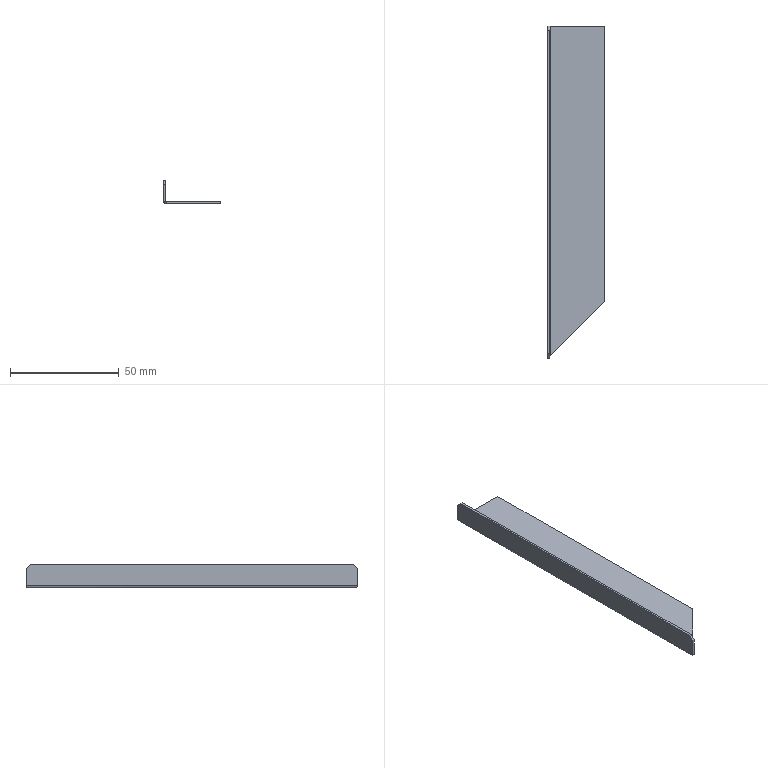Part | SolidWorks | features Chamfer 1, SplitBody 1 | 1 solid | 16 faces | box 26 x 152.414 x 11 mm | volume 5106 mm3 | plane 13 | cylinder 2 | spline 1 | commonest cylinder face diameters 0.2 x1 2.2 x1
STEP:
#1=CARTESIAN_POINT('',(-547.9,348.,56.));
#2=VERTEX_POINT('',#1);
#3=CARTESIAN_POINT('',(-547.9,348.,55.));
#4=VERTEX_POINT('',#3);
#5=CARTESIAN_POINT('',(-547.9,348.,56.));
#6=DIRECTION('',(0.,0.,-1.));
#7=VECTOR('',#6,1000.);
#8=LINE('',#5,#7);
#9=EDGE_CURVE('',#2,#4,#8,.T.);
#10=ORIENTED_EDGE('',*,*,#9,.F.);
#11=CARTESIAN_POINT('',(-523.,348.,56.));
#12=VERTEX_POINT('',#11);
#13=CARTESIAN_POINT('',(-549.,348.,56.));
#14=DIRECTION('',(1.,0.,0.));
#15=VECTOR('',#14,1000.);
#16=LINE('',#13,#15);
#17=EDGE_CURVE('',#2,#12,#16,.T.);
#18=ORIENTED_EDGE('',*,*,#17,.T.);
#19=CARTESIAN_POINT('',(-523.,348.,55.));
#20=VERTEX_POINT('',#19);
#21=CARTESIAN_POINT('',(-523.,348.,56.));
#22=DIRECTION('',(0.,0.,-1.));
#23=VECTOR('',#22,1000.);
#24=LINE('',#21,#23);
#25=EDGE_CURVE('',#12,#20,#24,.T.);
#26=ORIENTED_EDGE('',*,*,#25,.T.);
#27=CARTESIAN_POINT('',(-549.,348.,55.));
#28=DIRECTION('',(1.,0.,0.));
#29=VECTOR('',#28,1000.);
#30=LINE('',#27,#29);
#31=EDGE_CURVE('',#4,#20,#30,.T.);
#32=ORIENTED_EDGE('',*,*,#31,.F.);
#33=EDGE_LOOP('',(#10,#18,#26,#32));
#34=FACE_OUTER_BOUND('',#33,.T.);
#35=CARTESIAN_POINT('',(-549.,348.,56.));
#36=DIRECTION('',(0.,-1.,0.));
#37=DIRECTION('',(0.,0.,1.));
#38=AXIS2_PLACEMENT_3D('',#35,#36,#37);
#39=PLANE('',#38);
#40=ADVANCED_FACE('',(#34),#39,.F.);
#41=CARTESIAN_POINT('',(-547.9,196.686,56.));
#42=VERTEX_POINT('',#41);
#43=CARTESIAN_POINT('',(-547.9,196.686,55.));
#44=VERTEX_POINT('',#43);
#45=CARTESIAN_POINT('',(-547.9,196.686,56.));
#46=DIRECTION('',(0.,0.,-1.));
#47=VECTOR('',#46,1000.);
#48=LINE('',#45,#47);
#49=EDGE_CURVE('',#42,#44,#48,.T.);
#50=ORIENTED_EDGE('',*,*,#49,.T.);
#51=CARTESIAN_POINT('',(-523.,221.586,55.));
#52=VERTEX_POINT('',#51);
#53=CARTESIAN_POINT('',(-523.,221.586,55.));
#54=DIRECTION('',(-0.7071,-0.7071,0.));
#55=VECTOR('',#54,1000.);
#56=LINE('',#53,#55);
#57=EDGE_CURVE('',#52,#44,#56,.T.);
#58=ORIENTED_EDGE('',*,*,#57,.F.);
#59=CARTESIAN_POINT('',(-523.,221.586,56.));
#60=VERTEX_POINT('',#59);
#61=CARTESIAN_POINT('',(-523.,221.586,56.));
#62=DIRECTION('',(0.,0.,-1.));
#63=VECTOR('',#62,1000.);
#64=LINE('',#61,#63);
#65=EDGE_CURVE('',#60,#52,#64,.T.);
#66=ORIENTED_EDGE('',*,*,#65,.F.);
#67=CARTESIAN_POINT('',(-523.,221.586,56.));
#68=DIRECTION('',(-0.7071,-0.7071,0.));
#69=VECTOR('',#68,1000.);
#70=LINE('',#67,#69);
#71=EDGE_CURVE('',#60,#42,#70,.T.);
#72=ORIENTED_EDGE('',*,*,#71,.T.);
#73=EDGE_LOOP('',(#50,#58,#66,#72));
#74=FACE_OUTER_BOUND('',#73,.T.);
#75=CARTESIAN_POINT('',(-523.,221.586,56.));
#76=DIRECTION('',(-0.7071,0.7071,0.));
#77=DIRECTION('',(-0.7071,-0.7071,0.));
#78=AXIS2_PLACEMENT_3D('',#75,#76,#77);
#79=PLANE('',#78);
#80=ADVANCED_FACE('',(#74),#79,.F.);
#81=ORIENTED_EDGE('',*,*,#71,.F.);
#82=CARTESIAN_POINT('',(-523.,348.,56.));
#83=DIRECTION('',(0.,-1.,0.));
#84=VECTOR('',#83,1000.);
#85=LINE('',#82,#84);
#86=EDGE_CURVE('',#12,#60,#85,.T.);
#87=ORIENTED_EDGE('',*,*,#86,.F.);
#88=ORIENTED_EDGE('',*,*,#17,.F.);
#89=CARTESIAN_POINT('',(-547.9,348.,56.));
#90=DIRECTION('',(0.,-1.,0.));
#91=VECTOR('',#90,1000.);
#92=LINE('',#89,#91);
#93=EDGE_CURVE('',#2,#42,#92,.T.);
#94=ORIENTED_EDGE('',*,*,#93,.T.);
#95=EDGE_LOOP('',(#81,#87,#88,#94));
#96=FACE_OUTER_BOUND('',#95,.T.);
#97=CARTESIAN_POINT('',(0.,0.,56.));
#98=DIRECTION('',(0.,0.,1.));
#99=DIRECTION('',(0.,1.,0.));
#100=AXIS2_PLACEMENT_3D('',#97,#98,#99);
#101=PLANE('',#100);
#102=ADVANCED_FACE('',(#96),#101,.T.);
#103=CARTESIAN_POINT('',(-547.9,348.,55.));
#104=DIRECTION('',(0.,-1.,0.));
#105=VECTOR('',#104,1000.);
#106=LINE('',#103,#105);
#107=EDGE_CURVE('',#4,#44,#106,.T.);
#108=ORIENTED_EDGE('',*,*,#107,.F.);
#109=ORIENTED_EDGE('',*,*,#31,.T.);
#110=CARTESIAN_POINT('',(-523.,348.,55.));
#111=DIRECTION('',(0.,-1.,0.));
#112=VECTOR('',#111,1000.);
#113=LINE('',#110,#112);
#114=EDGE_CURVE('',#20,#52,#113,.T.);
#115=ORIENTED_EDGE('',*,*,#114,.T.);
#116=ORIENTED_EDGE('',*,*,#57,.T.);
#117=EDGE_LOOP('',(#108,#109,#115,#116));
#118=FACE_OUTER_BOUND('',#117,.T.);
#119=CARTESIAN_POINT('',(0.,0.,55.));
#120=DIRECTION('',(0.,0.,1.));
#121=DIRECTION('',(0.,1.,0.));
#122=AXIS2_PLACEMENT_3D('',#119,#120,#121);
#123=PLANE('',#122);
#124=ADVANCED_FACE('',(#118),#123,.F.);
#125=ORIENTED_EDGE('',*,*,#114,.F.);
#126=ORIENTED_EDGE('',*,*,#25,.F.);
#127=ORIENTED_EDGE('',*,*,#86,.T.);
#128=ORIENTED_EDGE('',*,*,#65,.T.);
#129=EDGE_LOOP('',(#125,#126,#127,#128));
#130=FACE_OUTER_BOUND('',#129,.T.);
#131=CARTESIAN_POINT('',(-523.,348.,56.));
#132=DIRECTION('',(-1.,0.,0.));
#133=DIRECTION('',(0.,0.,-1.));
#134=AXIS2_PLACEMENT_3D('',#131,#132,#133);
#135=PLANE('',#134);
#136=ADVANCED_FACE('',(#130),#135,.F.);
#137=CARTESIAN_POINT('',(-548.,195.586,56.1));
#138=VERTEX_POINT('',#137);
#139=CARTESIAN_POINT('',(-549.,195.586,56.1));
#140=VERTEX_POINT('',#139);
#141=CARTESIAN_POINT('',(-549.,195.586,56.1));
#142=DIRECTION('',(-1.,0.,0.));
#143=VECTOR('',#142,1000.);
#144=LINE('',#141,#143);
#145=EDGE_CURVE('',#138,#140,#144,.T.);
#146=ORIENTED_EDGE('',*,*,#145,.T.);
#147=CARTESIAN_POINT('',(-547.9,196.686,55.));
#148=CARTESIAN_POINT('',(-548.191,196.501,55.));
#149=CARTESIAN_POINT('',(-548.473,196.32,55.117));
#150=CARTESIAN_POINT('',(-548.781,196.043,55.425));
#151=CARTESIAN_POINT('',(-548.861,195.953,55.545));
#152=CARTESIAN_POINT('',(-548.972,195.768,55.813));
#153=CARTESIAN_POINT('',(-549.,195.678,55.955));
#154=CARTESIAN_POINT('',(-549.,195.586,56.1));
#155=B_SPLINE_CURVE_WITH_KNOTS('',3,(#147,#148,#149,#150,#151,#152,#153,#154),.UNSPECIFIED.,.F.,.F.,(4,2,2,4),(0.,0.001021,0.001531,0.002041),.UNSPECIFIED.);
#156=EDGE_CURVE('',#44,#140,#155,.T.);
#157=ORIENTED_EDGE('',*,*,#156,.F.);
#158=ORIENTED_EDGE('',*,*,#49,.F.);
#159=CARTESIAN_POINT('',(-547.9,196.686,56.));
#160=CARTESIAN_POINT('',(-547.926,196.502,56.));
#161=CARTESIAN_POINT('',(-547.952,196.319,56.011));
#162=CARTESIAN_POINT('',(-547.989,195.952,56.048));
#163=CARTESIAN_POINT('',(-548.,195.769,56.074));
#164=CARTESIAN_POINT('',(-548.,195.586,56.1));
#165=B_SPLINE_CURVE_WITH_KNOTS('',3,(#159,#160,#161,#162,#163,#164),.UNSPECIFIED.,.F.,.F.,(4,2,4),(0.,0.5,1.),.UNSPECIFIED.);
#166=EDGE_CURVE('',#42,#138,#165,.T.);
#167=ORIENTED_EDGE('',*,*,#166,.T.);
#168=EDGE_LOOP('',(#146,#157,#158,#167));
#169=FACE_OUTER_BOUND('',#168,.T.);
#170=CARTESIAN_POINT('',(-547.9,196.686,54.99));
#171=CARTESIAN_POINT('',(-548.045,196.594,54.99));
#172=CARTESIAN_POINT('',(-548.191,196.502,55.019));
#173=CARTESIAN_POINT('',(-548.459,196.319,55.13));
#174=CARTESIAN_POINT('',(-548.582,196.227,55.212));
#175=CARTESIAN_POINT('',(-548.788,196.044,55.418));
#176=CARTESIAN_POINT('',(-548.87,195.952,55.541));
#177=CARTESIAN_POINT('',(-548.981,195.769,55.809));
#178=CARTESIAN_POINT('',(-549.01,195.677,55.955));
#179=CARTESIAN_POINT('',(-549.01,195.586,56.1));
#180=CARTESIAN_POINT('',(-547.9,196.686,55.));
#181=CARTESIAN_POINT('',(-548.044,196.594,55.));
#182=CARTESIAN_POINT('',(-548.188,196.502,55.029));
#183=CARTESIAN_POINT('',(-548.454,196.319,55.139));
#184=CARTESIAN_POINT('',(-548.576,196.227,55.22));
#185=CARTESIAN_POINT('',(-548.78,196.044,55.424));
#186=CARTESIAN_POINT('',(-548.861,195.952,55.546));
#187=CARTESIAN_POINT('',(-548.971,195.769,55.812));
#188=CARTESIAN_POINT('',(-549.,195.677,55.956));
#189=CARTESIAN_POINT('',(-549.,195.586,56.1));
#190=CARTESIAN_POINT('',(-547.9,196.686,56.));
#191=CARTESIAN_POINT('',(-547.913,196.594,56.));
#192=CARTESIAN_POINT('',(-547.926,196.502,56.003));
#193=CARTESIAN_POINT('',(-547.95,196.319,56.013));
#194=CARTESIAN_POINT('',(-547.961,196.227,56.02));
#195=CARTESIAN_POINT('',(-547.98,196.044,56.039));
#196=CARTESIAN_POINT('',(-547.987,195.952,56.05));
#197=CARTESIAN_POINT('',(-547.997,195.769,56.074));
#198=CARTESIAN_POINT('',(-548.,195.677,56.087));
#199=CARTESIAN_POINT('',(-548.,195.586,56.1));
#200=B_SPLINE_SURFACE_WITH_KNOTS('',1,3,((#170,#171,#172,#173,#174,#175,#176,#177,#178,#179),(#180,#181,#182,#183,#184,#185,#186,#187,#188,#189),(#190,#191,#192,#193,#194,#195,#196,#197,#198,#199)),.UNSPECIFIED.,.F.,.F.,.F.,(2,1,2),(4,2,2,2,4),(-0.01,0.,1.),(0.,0.25,0.5,0.75,1.),.UNSPECIFIED.);
#201=ADVANCED_FACE('',(#169),#200,.T.);
#202=CARTESIAN_POINT('',(-548.,348.,56.1));
#203=VERTEX_POINT('',#202);
#204=CARTESIAN_POINT('',(-547.9,348.,56.1));
#205=DIRECTION('',(0.,-1.,0.));
#206=DIRECTION('',(0.,0.,-1.));
#207=AXIS2_PLACEMENT_3D('',#204,#205,#206);
#208=CIRCLE('',#207,0.1);
#209=EDGE_CURVE('',#203,#2,#208,.T.);
#210=ORIENTED_EDGE('',*,*,#209,.T.);
#211=ORIENTED_EDGE('',*,*,#9,.T.);
#212=CARTESIAN_POINT('',(-549.,348.,56.1));
#213=VERTEX_POINT('',#212);
#214=CARTESIAN_POINT('',(-547.9,348.,56.1));
#215=DIRECTION('',(0.,-1.,0.));
#216=DIRECTION('',(0.,0.,-1.));
#217=AXIS2_PLACEMENT_3D('',#214,#215,#216);
#218=CIRCLE('',#217,1.1);
#219=EDGE_CURVE('',#213,#4,#218,.T.);
#220=ORIENTED_EDGE('',*,*,#219,.F.);
#221=CARTESIAN_POINT('',(-548.,348.,56.1));
#222=DIRECTION('',(-1.,0.,0.));
#223=VECTOR('',#222,1000.);
#224=LINE('',#221,#223);
#225=EDGE_CURVE('',#203,#213,#224,.T.);
#226=ORIENTED_EDGE('',*,*,#225,.F.);
#227=EDGE_LOOP('',(#210,#211,#220,#226));
#228=FACE_OUTER_BOUND('',#227,.T.);
#229=CARTESIAN_POINT('',(-547.9,348.,56.1));
#230=DIRECTION('',(0.,-1.,0.));
#231=DIRECTION('',(0.,0.,1.));
#232=AXIS2_PLACEMENT_3D('',#229,#230,#231);
#233=PLANE('',#232);
#234=ADVANCED_FACE('',(#228),#233,.F.);
#235=ORIENTED_EDGE('',*,*,#107,.T.);
#236=ORIENTED_EDGE('',*,*,#156,.T.);
#237=CARTESIAN_POINT('',(-549.,195.586,56.1));
#238=DIRECTION('',(0.,-1.,0.));
#239=VECTOR('',#238,1000.);
#240=LINE('',#237,#239);
#241=EDGE_CURVE('',#213,#140,#240,.T.);
#242=ORIENTED_EDGE('',*,*,#241,.F.);
#243=ORIENTED_EDGE('',*,*,#219,.T.);
#244=EDGE_LOOP('',(#235,#236,#242,#243));
#245=FACE_OUTER_BOUND('',#244,.T.);
#246=CARTESIAN_POINT('',(-547.9,348.,56.1));
#247=DIRECTION('',(0.,1.,0.));
#248=DIRECTION('',(-1.,0.,0.));
#249=AXIS2_PLACEMENT_3D('',#246,#247,#248);
#250=CYLINDRICAL_SURFACE('',#249,1.1);
#251=ADVANCED_FACE('',(#245),#250,.T.);
#252=ORIENTED_EDGE('',*,*,#93,.F.);
#253=ORIENTED_EDGE('',*,*,#209,.F.);
#254=CARTESIAN_POINT('',(-548.,195.586,56.1));
#255=DIRECTION('',(0.,1.,0.));
#256=VECTOR('',#255,1000.);
#257=LINE('',#254,#256);
#258=EDGE_CURVE('',#138,#203,#257,.T.);
#259=ORIENTED_EDGE('',*,*,#258,.F.);
#260=ORIENTED_EDGE('',*,*,#166,.F.);
#261=EDGE_LOOP('',(#252,#253,#259,#260));
#262=FACE_OUTER_BOUND('',#261,.T.);
#263=CARTESIAN_POINT('',(-547.9,348.,56.1));
#264=DIRECTION('',(0.,1.,0.));
#265=DIRECTION('',(-1.,0.,0.));
#266=AXIS2_PLACEMENT_3D('',#263,#264,#265);
#267=CYLINDRICAL_SURFACE('',#266,0.1);
#268=ADVANCED_FACE('',(#262),#267,.F.);
#269=CARTESIAN_POINT('',(-548.,195.586,64.));
#270=VERTEX_POINT('',#269);
#271=CARTESIAN_POINT('',(-548.,195.586,56.));
#272=DIRECTION('',(0.,0.,-1.));
#273=VECTOR('',#272,1000.);
#274=LINE('',#271,#273);
#275=EDGE_CURVE('',#270,#138,#274,.T.);
#276=ORIENTED_EDGE('',*,*,#275,.F.);
#277=CARTESIAN_POINT('',(-549.,195.586,64.));
#278=VERTEX_POINT('',#277);
#279=CARTESIAN_POINT('',(-549.,195.586,64.));
#280=DIRECTION('',(-1.,0.,0.));
#281=VECTOR('',#280,1000.);
#282=LINE('',#279,#281);
#283=EDGE_CURVE('',#270,#278,#282,.T.);
#284=ORIENTED_EDGE('',*,*,#283,.T.);
#285=CARTESIAN_POINT('',(-549.,195.586,-40.));
#286=DIRECTION('',(0.,0.,-1.));
#287=VECTOR('',#286,1000.);
#288=LINE('',#285,#287);
#289=EDGE_CURVE('',#278,#140,#288,.T.);
#290=ORIENTED_EDGE('',*,*,#289,.T.);
#291=ORIENTED_EDGE('',*,*,#145,.F.);
#292=EDGE_LOOP('',(#276,#284,#290,#291));
#293=FACE_OUTER_BOUND('',#292,.T.);
#294=CARTESIAN_POINT('',(-549.,195.586,56.));
#295=DIRECTION('',(0.,1.,0.));
#296=DIRECTION('',(-1.,0.,0.));
#297=AXIS2_PLACEMENT_3D('',#294,#295,#296);
#298=PLANE('',#297);
#299=ADVANCED_FACE('',(#293),#298,.F.);
#300=CARTESIAN_POINT('',(-549.,348.,64.));
#301=VERTEX_POINT('',#300);
#302=CARTESIAN_POINT('',(-549.,348.,-40.));
#303=DIRECTION('',(0.,0.,1.));
#304=VECTOR('',#303,1000.);
#305=LINE('',#302,#304);
#306=EDGE_CURVE('',#213,#301,#305,.T.);
#307=ORIENTED_EDGE('',*,*,#306,.T.);
#308=CARTESIAN_POINT('',(-548.,348.,64.));
#309=VERTEX_POINT('',#308);
#310=CARTESIAN_POINT('',(-549.,348.,64.));
#311=DIRECTION('',(1.,0.,0.));
#312=VECTOR('',#311,1000.);
#313=LINE('',#310,#312);
#314=EDGE_CURVE('',#301,#309,#313,.T.);
#315=ORIENTED_EDGE('',*,*,#314,.T.);
#316=CARTESIAN_POINT('',(-548.,348.,66.));
#317=DIRECTION('',(0.,0.,1.));
#318=VECTOR('',#317,1000.);
#319=LINE('',#316,#318);
#320=EDGE_CURVE('',#203,#309,#319,.T.);
#321=ORIENTED_EDGE('',*,*,#320,.F.);
#322=ORIENTED_EDGE('',*,*,#225,.T.);
#323=EDGE_LOOP('',(#307,#315,#321,#322));
#324=FACE_OUTER_BOUND('',#323,.T.);
#325=CARTESIAN_POINT('',(-549.,348.,66.));
#326=DIRECTION('',(0.,-1.,0.));
#327=DIRECTION('',(1.,0.,0.));
#328=AXIS2_PLACEMENT_3D('',#325,#326,#327);
#329=PLANE('',#328);
#330=ADVANCED_FACE('',(#324),#329,.F.);
#331=ORIENTED_EDGE('',*,*,#289,.F.);
#332=CARTESIAN_POINT('',(-549.,197.586,66.));
#333=VERTEX_POINT('',#332);
#334=CARTESIAN_POINT('',(-549.,197.586,66.));
#335=DIRECTION('',(0.,0.7071,0.7071));
#336=VECTOR('',#335,1000.);
#337=LINE('',#334,#336);
#338=EDGE_CURVE('',#278,#333,#337,.T.);
#339=ORIENTED_EDGE('',*,*,#338,.T.);
#340=CARTESIAN_POINT('',(-549.,346.,66.));
#341=VERTEX_POINT('',#340);
#342=CARTESIAN_POINT('',(-549.,0.,66.));
#343=DIRECTION('',(0.,-1.,0.));
#344=VECTOR('',#343,1000.);
#345=LINE('',#342,#344);
#346=EDGE_CURVE('',#341,#333,#345,.T.);
#347=ORIENTED_EDGE('',*,*,#346,.F.);
#348=CARTESIAN_POINT('',(-549.,348.,64.));
#349=DIRECTION('',(0.,0.7071,-0.7071));
#350=VECTOR('',#349,1000.);
#351=LINE('',#348,#350);
#352=EDGE_CURVE('',#341,#301,#351,.T.);
#353=ORIENTED_EDGE('',*,*,#352,.T.);
#354=ORIENTED_EDGE('',*,*,#306,.F.);
#355=ORIENTED_EDGE('',*,*,#241,.T.);
#356=EDGE_LOOP('',(#331,#339,#347,#353,#354,#355));
#357=FACE_OUTER_BOUND('',#356,.T.);
#358=CARTESIAN_POINT('',(-549.,0.,-40.));
#359=DIRECTION('',(1.,0.,0.));
#360=DIRECTION('',(0.,0.,1.));
#361=AXIS2_PLACEMENT_3D('',#358,#359,#360);
#362=PLANE('',#361);
#363=ADVANCED_FACE('',(#357),#362,.F.);
#364=CARTESIAN_POINT('',(-548.,346.,66.));
#365=VERTEX_POINT('',#364);
#366=CARTESIAN_POINT('',(-548.,197.586,66.));
#367=VERTEX_POINT('',#366);
#368=CARTESIAN_POINT('',(-548.,195.586,66.));
#369=DIRECTION('',(0.,-1.,0.));
#370=VECTOR('',#369,1000.);
#371=LINE('',#368,#370);
#372=EDGE_CURVE('',#365,#367,#371,.T.);
#373=ORIENTED_EDGE('',*,*,#372,.T.);
#374=CARTESIAN_POINT('',(-548.,45.793,-85.793));
#375=DIRECTION('',(0.,-0.7071,-0.7071));
#376=VECTOR('',#375,1000.);
#377=LINE('',#374,#376);
#378=EDGE_CURVE('',#367,#270,#377,.T.);
#379=ORIENTED_EDGE('',*,*,#378,.T.);
#380=ORIENTED_EDGE('',*,*,#275,.T.);
#381=ORIENTED_EDGE('',*,*,#258,.T.);
#382=ORIENTED_EDGE('',*,*,#320,.T.);
#383=CARTESIAN_POINT('',(-548.,226.,186.));
#384=DIRECTION('',(0.,-0.7071,0.7071));
#385=VECTOR('',#384,1000.);
#386=LINE('',#383,#385);
#387=EDGE_CURVE('',#309,#365,#386,.T.);
#388=ORIENTED_EDGE('',*,*,#387,.T.);
#389=EDGE_LOOP('',(#373,#379,#380,#381,#382,#388));
#390=FACE_OUTER_BOUND('',#389,.T.);
#391=CARTESIAN_POINT('',(-548.,0.,-40.));
#392=DIRECTION('',(1.,0.,0.));
#393=DIRECTION('',(0.,0.,1.));
#394=AXIS2_PLACEMENT_3D('',#391,#392,#393);
#395=PLANE('',#394);
#396=ADVANCED_FACE('',(#390),#395,.T.);
#397=ORIENTED_EDGE('',*,*,#346,.T.);
#398=CARTESIAN_POINT('',(-549.,197.586,66.));
#399=DIRECTION('',(1.,0.,0.));
#400=VECTOR('',#399,1000.);
#401=LINE('',#398,#400);
#402=EDGE_CURVE('',#333,#367,#401,.T.);
#403=ORIENTED_EDGE('',*,*,#402,.T.);
#404=ORIENTED_EDGE('',*,*,#372,.F.);
#405=CARTESIAN_POINT('',(-549.,346.,66.));
#406=DIRECTION('',(-1.,0.,0.));
#407=VECTOR('',#406,1000.);
#408=LINE('',#405,#407);
#409=EDGE_CURVE('',#365,#341,#408,.T.);
#410=ORIENTED_EDGE('',*,*,#409,.T.);
#411=EDGE_LOOP('',(#397,#403,#404,#410));
#412=FACE_OUTER_BOUND('',#411,.T.);
#413=CARTESIAN_POINT('',(-549.,195.586,66.));
#414=DIRECTION('',(0.,0.,-1.));
#415=DIRECTION('',(1.,0.,0.));
#416=AXIS2_PLACEMENT_3D('',#413,#414,#415);
#417=PLANE('',#416);
#418=ADVANCED_FACE('',(#412),#417,.F.);
#419=ORIENTED_EDGE('',*,*,#338,.F.);
#420=ORIENTED_EDGE('',*,*,#283,.F.);
#421=ORIENTED_EDGE('',*,*,#378,.F.);
#422=ORIENTED_EDGE('',*,*,#402,.F.);
#423=EDGE_LOOP('',(#419,#420,#421,#422));
#424=FACE_OUTER_BOUND('',#423,.T.);
#425=CARTESIAN_POINT('',(-549.,197.586,66.));
#426=DIRECTION('',(0.,0.7071,-0.7071));
#427=DIRECTION('',(1.,0.,0.));
#428=AXIS2_PLACEMENT_3D('',#425,#426,#427);
#429=PLANE('',#428);
#430=ADVANCED_FACE('',(#424),#429,.F.);
#431=ORIENTED_EDGE('',*,*,#352,.F.);
#432=ORIENTED_EDGE('',*,*,#409,.F.);
#433=ORIENTED_EDGE('',*,*,#387,.F.);
#434=ORIENTED_EDGE('',*,*,#314,.F.);
#435=EDGE_LOOP('',(#431,#432,#433,#434));
#436=FACE_OUTER_BOUND('',#435,.T.);
#437=CARTESIAN_POINT('',(-549.,348.,64.));
#438=DIRECTION('',(0.,-0.7071,-0.7071));
#439=DIRECTION('',(1.,0.,0.));
#440=AXIS2_PLACEMENT_3D('',#437,#438,#439);
#441=PLANE('',#440);
#442=ADVANCED_FACE('',(#436),#441,.F.);
#443=CLOSED_SHELL('',(#40,#80,#102,#124,#136,#201,#234,#251,#268,#299,#330,#363,#396,#418,#430,#442));
#444=MANIFOLD_SOLID_BREP('',#443);
#445=CARTESIAN_POINT('',(0.,0.,0.));
#446=DIRECTION('',(0.,0.,1.));
#447=DIRECTION('',(1.,0.,0.));
#448=AXIS2_PLACEMENT_3D('',#445,#446,#447);
#449=(LENGTH_UNIT()NAMED_UNIT(*)SI_UNIT(.MILLI.,.METRE.));
#450=UNCERTAINTY_MEASURE_WITH_UNIT(LENGTH_MEASURE(0.00001),#449,'','');
#451=(NAMED_UNIT(*)PLANE_ANGLE_UNIT()SI_UNIT($,.RADIAN.));
#452=(NAMED_UNIT(*)SI_UNIT($,.STERADIAN.)SOLID_ANGLE_UNIT());
#453=(GEOMETRIC_REPRESENTATION_CONTEXT(3)GLOBAL_UNCERTAINTY_ASSIGNED_CONTEXT((#450))GLOBAL_UNIT_ASSIGNED_CONTEXT((#449,#451,#452))REPRESENTATION_CONTEXT('',''));
#454=ADVANCED_BREP_SHAPE_REPRESENTATION('',(#444,#448),#453);